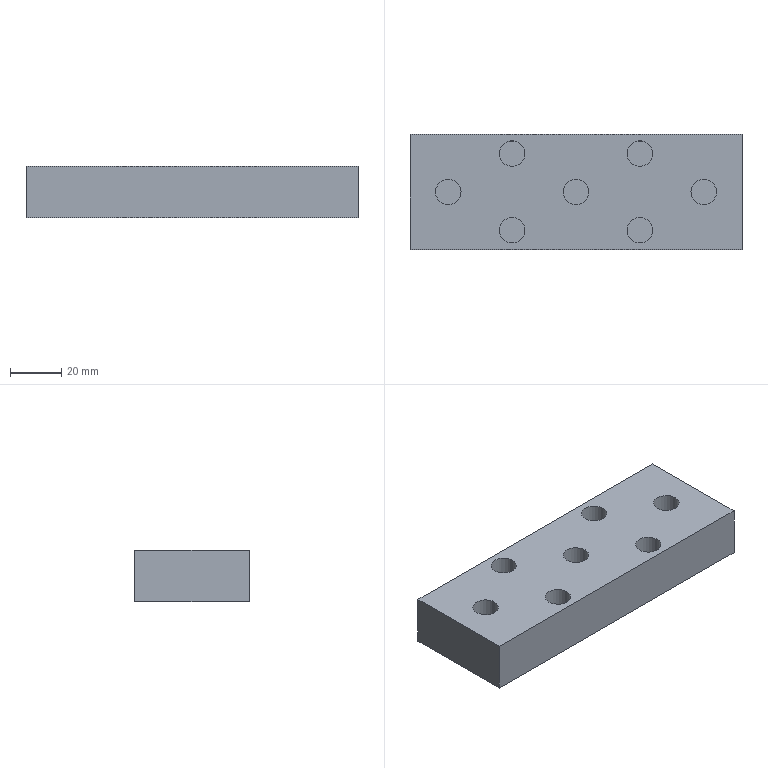NC program | NX | posted with a generic post | part box 130 x 45 x 20 mm
Lines 3396 to 3690 of 3690:
(PLANAR_MILL_1_COPY , TOOL : D8精光)
N6766 T10 M6
N6768 G54
N6770 G17 G0 G90 X24.803 Y-15.465 S4500 M3
N6772 G43 Z30. H10
N6774 Z-8.
N6776 G94 G1 Z-10. F600.
N6778 G41 X25. Y-15.5 D10
N6780 X25.5
N6782 G3 X26. Y-15. R0.5
N6784 X25. Y-14. R1.
N6786 X26. Y-15. R-1.
N6788 X25.5 Y-14.5 R0.5
N6790 G40
N6792 G1 X25.303 Y-14.535
N6794 Y-15.465
N6796 G41 X25.5 Y-15.5
N6798 G3 X26. Y-15. R0.5
N6800 X25. Y-14. R1.
N6802 X26. Y-15. R-1.
N6804 X25.5 Y-14.5 R0.5
N6806 G1 X25.
N6808 G40
N6810 X24.803 Y-14.535
N6812 Z-8.
N6814 G0 Z30.
N6816 X49.803 Y-0.465
N6818 Z-8.
N6820 G1 Z-10.
N6822 G41 X50. Y-0.5
N6824 X50.5
N6826 G3 X51. Y0. R0.5
N6828 X50. Y1. R1.
N6830 X51. Y0. R-1.
N6832 X50.5 Y0.5 R0.5
N6834 G40
N6836 G1 X50.303 Y0.465
N6838 Y-0.465
N6840 G41 X50.5 Y-0.5
N6842 G3 X51. Y0. R0.5
N6844 X50. Y1. R1.
N6846 X51. Y0. R-1.
N6848 X50.5 Y0.5 R0.5
N6850 G1 X50.
N6852 G40
N6854 X49.803 Y0.465
N6856 Z-8.
N6858 G0 Z30.
N6860 X24.803 Y14.535
N6862 Z-8.
N6864 G1 Z-10.
N6866 G41 X25. Y14.5
N6868 X25.5
N6870 G3 X26. Y15. R0.5
N6872 X25. Y16. R1.
N6874 X26. Y15. R-1.
N6876 X25.5 Y15.5 R0.5
N6878 G40
N6880 G1 X25.303 Y15.465
N6882 Y14.535
N6884 G41 X25.5 Y14.5
N6886 G3 X26. Y15. R0.5
N6888 X25. Y16. R1.
N6890 X26. Y15. R-1.
N6892 X25.5 Y15.5 R0.5
N6894 G1 X25.
N6896 G40
N6898 X24.803 Y15.465
N6900 Z-8.
N6902 G0 Z30.
N6904 X-0.197 Y-0.465
N6906 Z-8.
N6908 G1 Z-10.
N6910 G41 X0. Y-0.5
N6912 X0.5
N6914 G3 X1. Y0. R0.5
N6916 X0. Y1. R1.
N6918 X1. Y0. R-1.
N6920 X0.5 Y0.5 R0.5
N6922 G40
N6924 G1 X0.303 Y0.465
N6926 Y-0.465
N6928 G41 X0.5 Y-0.5
N6930 G3 X1. Y0. R0.5
N6932 X0. Y1. R1.
N6934 X1. Y0. R-1.
N6936 X0.5 Y0.5 R0.5
N6938 G40
N6940 G1 X0.354 Y0.354
N6942 Z-8.
N6944 G0 Z30.
N6946 X-25.197 Y14.535
N6948 Z-8.
N6950 G1 Z-10.
N6952 G41 X-25. Y14.5
N6954 X-24.5
N6956 G3 X-24. Y15. R0.5
N6958 X-25. Y16. R1.
N6960 X-24. Y15. R-1.
N6962 X-24.5 Y15.5 R0.5
N6964 G40
N6966 G1 X-24.697 Y15.465
N6968 Y14.535
N6970 G41 X-24.5 Y14.5
N6972 G3 X-24. Y15. R0.5
N6974 X-25. Y16. R1.
N6976 X-24. Y15. R-1.
N6978 X-24.5 Y15.5 R0.5
N6980 G1 X-25.
N6982 G40
N6984 X-25.197 Y15.465
N6986 Z-8.
N6988 G0 Z30.
N6990 X-50.197 Y-0.465
N6992 Z-8.
N6994 G1 Z-10.
N6996 G41 X-50. Y-0.5
N6998 X-49.5
N7000 G3 X-49. Y0. R0.5
N7002 X-50. Y1. R1.
N7004 X-49. Y0. R-1.
N7006 X-49.5 Y0.5 R0.5
N7008 G40
N7010 G1 X-49.697 Y0.465
N7012 Y-0.465
N7014 G41 X-49.5 Y-0.5
N7016 G3 X-49. Y0. R0.5
N7018 X-50. Y1. R1.
N7020 X-49. Y0. R-1.
N7022 X-49.5 Y0.5 R0.5
N7024 G1 X-50.
N7026 G40
N7028 X-50.197 Y0.465
N7030 Z-8.
N7032 G0 Z30.
N7034 X-25.197 Y-15.465
N7036 Z-8.
N7038 G1 Z-10.
N7040 G41 X-25. Y-15.5
N7042 X-24.5
N7044 G3 X-24. Y-15. R0.5
N7046 X-25. Y-14. R1.
N7048 X-24. Y-15. R-1.
N7050 X-24.5 Y-14.5 R0.5
N7052 G40
N7054 G1 X-24.697 Y-14.535
N7056 Y-15.465
N7058 G41 X-24.5 Y-15.5
N7060 G3 X-24. Y-15. R0.5
N7062 X-25. Y-14. R1.
N7064 X-24. Y-15. R-1.
N7066 X-24.5 Y-14.5 R0.5
N7068 G1 X-25.
N7070 G40
N7072 X-25.197 Y-14.535
N7074 Z-8.
N7076 G0 Z30.
(PLANAR_MILL_2 , TOOL : D8精光)
N7078 X-69. Y-29.428
N7080 Z-17.
N7082 G1 Z-20.
N7084 Y-22.498
N7086 Y22.5
N7088 G2 X-65. Y26.5 R4.
N7090 G1 X65.
N7092 G2 X69. Y22.5 R4.
N7094 G1 Y-22.5
N7096 G2 X65. Y-26.5 R4.
N7098 G1 X-64.998
N7100 X-71.928
N7102 Z-17.
N7104 G0 Z30.
N7106 M5
(PLANAR_MILL_1_COPY_COPY , TOOL : D10点钻)
N7108 T02 M6
N7110 G54
N7112 G17 G0 G90 X27.862 Y-15.465 S3500 M3
N7114 G43 Z30. H2
N7116 Z0.5
N7118 G94 G1 Z-1.5 F800.
N7120 G41 X28.059 Y-15.5 D2
N7122 X28.1
N7124 G3 X28.6 Y-15. R0.5
N7126 X25. Y-11.4 R3.6
N7128 X28.6 Y-15. R-3.6
N7130 X28.059 Y-14.5 R0.502
N7132 G40
N7134 G1 X27.862 Y-14.535
N7136 Z0.5
N7138 G0 Z30.
N7140 X52.862 Y-0.465
N7142 Z0.5
N7144 G1 Z-1.5
N7146 G41 X53.059 Y-0.5
N7148 X53.1
N7150 G3 X53.6 Y0. R0.5
N7152 X50. Y3.6 R3.6
N7154 X53.6 Y0. R-3.6
N7156 X53.059 Y0.5 R0.502
N7158 G40
N7160 G1 X52.862 Y0.465
N7162 Z0.5
N7164 G0 Z30.
N7166 X27.862 Y14.535
N7168 Z0.5
N7170 G1 Z-1.5
N7172 G41 X28.059 Y14.5
N7174 X28.1
N7176 G3 X28.6 Y15. R0.5
N7178 X25. Y18.6 R3.6
N7180 X28.6 Y15. R-3.6
N7182 X28.059 Y15.5 R0.502
N7184 G40
N7186 G1 X27.862 Y15.465
N7188 Z0.5
N7190 G0 Z30.
N7192 X2.862 Y-0.465
N7194 Z0.5
N7196 G1 Z-1.5
N7198 G41 X3.059 Y-0.5
N7200 X3.1
N7202 G3 X3.6 Y0. R0.5
N7204 X0. Y3.6 R3.6
N7206 X3.6 Y0. R-3.6
N7208 X3.059 Y0.5 R0.502
N7210 G40
N7212 G1 X2.862 Y0.465
N7214 Z0.5
N7216 G0 Z30.
N7218 X-22.138 Y14.535
N7220 Z0.5
N7222 G1 Z-1.5
N7224 G41 X-21.941 Y14.5
N7226 X-21.9
N7228 G3 X-21.4 Y15. R0.5
N7230 X-25. Y18.6 R3.6
N7232 X-21.4 Y15. R-3.6
N7234 X-21.941 Y15.5 R0.502
N7236 G40
N7238 G1 X-22.138 Y15.465
N7240 Z0.5
N7242 G0 Z30.
N7244 X-47.138 Y-0.465
N7246 Z0.5
N7248 G1 Z-1.5
N7250 G41 X-46.941 Y-0.5
N7252 X-46.9
N7254 G3 X-46.4 Y0. R0.5
N7256 X-50. Y3.6 R3.6
N7258 X-46.4 Y0. R-3.6
N7260 X-46.941 Y0.5 R0.502
N7262 G40
N7264 G1 X-47.138 Y0.465
N7266 Z0.5
N7268 G0 Z30.
N7270 X-22.138 Y-15.465
N7272 Z0.5
N7274 G1 Z-1.5
N7276 G41 X-21.941 Y-15.5
N7278 X-21.9
N7280 G3 X-21.4 Y-15. R0.5
N7282 X-25. Y-11.4 R3.6
N7284 X-21.4 Y-15. R-3.6
N7286 X-21.941 Y-14.5 R0.502
N7288 G40
N7290 G1 X-22.138 Y-14.535
N7292 Z0.5
N7294 G0 Z30.
(PLANAR_MILL_2_COPY , TOOL : D10点钻)
N7296 X0. Y28.9
N7298 Z1.5
N7300 G1 Z-1.5
N7302 Y23.9
N7304 X64.9
N7306 G2 X66.4 Y22.4 R1.5
N7308 G1 Y-22.4
N7310 G2 X64.9 Y-23.9 R1.5
N7312 G1 X-64.9
N7314 G2 X-66.4 Y-22.4 R1.5
N7316 G1 Y22.4
N7318 G2 X-64.9 Y23.9 R1.5
N7320 G1 X0.
N7322 Y28.9
N7324 Z1.5
N7326 G0 Z30.
N7328 M5
N7330 M2